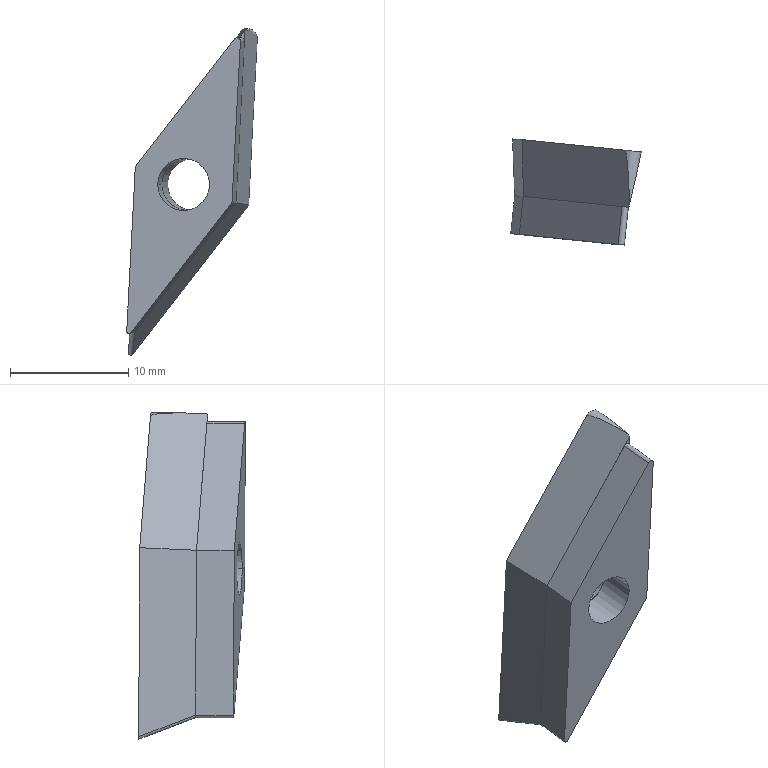Part | Mastercam | 2 solids | 20 faces | box 11.025 x 9.006 x 27.564 mm | volume 930.962 mm3 | plane 12 | cylinder 7 | spline 1 | commonest cylinder face diameters 4.4 x4 0.4 x1 0.6 x1 1.6 x1
STEP:
#1=CARTESIAN_POINT('',(0.,0.,0.));
#2=DIRECTION('',(0.,0.,1.));
#3=DIRECTION('',(1.,0.,0.));
#4=AXIS2_PLACEMENT_3D('',#1,#2,#3);
#5=CARTESIAN_POINT('',(13.05,0.4403,29.477));
#6=VERTEX_POINT('',#5);
#7=CARTESIAN_POINT('',(13.266,0.4177,26.373));
#8=VERTEX_POINT('',#7);
#9=CARTESIAN_POINT('',(11.614,0.5912,27.817));
#10=DIRECTION('',(0.1045,0.9945,0.));
#11=DIRECTION('',(0.7506,-0.07889,-0.6561));
#12=AXIS2_PLACEMENT_3D('',#9,#10,#11);
#13=CIRCLE('',#12,2.2);
#14=EDGE_CURVE('',#6,#8,#13,.T.);
#15=ORIENTED_EDGE('',*,*,#14,.F.);
#16=CARTESIAN_POINT('',(10.179,0.7421,26.156));
#17=VERTEX_POINT('',#16);
#18=CARTESIAN_POINT('',(11.614,0.5912,27.817));
#19=DIRECTION('',(0.1045,0.9945,0.));
#20=DIRECTION('',(0.7506,-0.07889,-0.6561));
#21=AXIS2_PLACEMENT_3D('',#18,#19,#20);
#22=CIRCLE('',#21,2.2);
#23=EDGE_CURVE('',#17,#6,#22,.T.);
#24=ORIENTED_EDGE('',*,*,#23,.F.);
#25=CARTESIAN_POINT('',(11.614,0.5912,27.817));
#26=DIRECTION('',(0.1045,0.9945,0.));
#27=DIRECTION('',(0.7506,-0.07889,-0.6561));
#28=AXIS2_PLACEMENT_3D('',#25,#26,#27);
#29=CIRCLE('',#28,2.2);
#30=EDGE_CURVE('',#8,#17,#29,.T.);
#31=ORIENTED_EDGE('',*,*,#30,.F.);
#32=EDGE_LOOP('',(#15,#24,#31));
#33=FACE_BOUND('',#32,.T.);
#34=CARTESIAN_POINT('',(16.266,0.1023,26.068));
#35=VERTEX_POINT('',#34);
#36=CARTESIAN_POINT('',(6.484,1.13,13.478));
#37=VERTEX_POINT('',#36);
#38=CARTESIAN_POINT('',(24.134,-0.7247,36.194));
#39=DIRECTION('',(-0.6123,0.06435,-0.788));
#40=VECTOR('',#39,1.);
#41=LINE('',#38,#40);
#42=EDGE_CURVE('',#35,#37,#41,.T.);
#43=ORIENTED_EDGE('',*,*,#42,.T.);
#44=CARTESIAN_POINT('',(6.131,1.168,13.611));
#45=VERTEX_POINT('',#44);
#46=CARTESIAN_POINT('',(6.332,1.146,13.609));
#47=DIRECTION('',(0.1045,0.9945,0.));
#48=DIRECTION('',(-0.3483,0.03661,-0.9367));
#49=AXIS2_PLACEMENT_3D('',#46,#47,#48);
#50=ELLIPSE('',#49,0.216,0.2);
#51=EDGE_CURVE('',#37,#45,#50,.T.);
#52=ORIENTED_EDGE('',*,*,#51,.T.);
#53=CARTESIAN_POINT('',(6.963,1.08,29.565));
#54=VERTEX_POINT('',#53);
#55=CARTESIAN_POINT('',(7.647,1.008,42.694));
#56=DIRECTION('',(-0.05205,0.005471,-0.9986));
#57=VECTOR('',#56,1.);
#58=LINE('',#55,#57);
#59=EDGE_CURVE('',#54,#45,#58,.T.);
#60=ORIENTED_EDGE('',*,*,#59,.F.);
#61=CARTESIAN_POINT('',(15.577,0.1747,40.652));
#62=VERTEX_POINT('',#61);
#63=CARTESIAN_POINT('',(16.67,0.05986,42.059));
#64=DIRECTION('',(0.6123,-0.06435,0.788));
#65=VECTOR('',#64,1.);
#66=LINE('',#63,#65);
#67=EDGE_CURVE('',#54,#62,#66,.T.);
#68=ORIENTED_EDGE('',*,*,#67,.T.);
#69=CARTESIAN_POINT('',(16.998,0.02532,40.118));
#70=VERTEX_POINT('',#69);
#71=CARTESIAN_POINT('',(16.204,0.1088,40.159));
#72=DIRECTION('',(-0.1045,-0.9945,0.));
#73=DIRECTION('',(0.6525,-0.06858,0.7547));
#74=AXIS2_PLACEMENT_3D('',#71,#72,#73);
#75=CIRCLE('',#74,0.8);
#76=EDGE_CURVE('',#70,#62,#75,.T.);
#77=ORIENTED_EDGE('',*,*,#76,.F.);
#78=CARTESIAN_POINT('',(17.107,0.01394,42.196));
#79=DIRECTION('',(0.05205,-0.005471,0.9986));
#80=VECTOR('',#79,1.);
#81=LINE('',#78,#80);
#82=EDGE_CURVE('',#35,#70,#81,.T.);
#83=ORIENTED_EDGE('',*,*,#82,.F.);
#84=EDGE_LOOP('',(#43,#52,#60,#68,#77,#83));
#85=FACE_OUTER_BOUND('',#84,.T.);
#86=CARTESIAN_POINT('',(16.451,0.08283,42.23));
#87=DIRECTION('',(-0.1045,-0.9945,0.));
#88=DIRECTION('',(-0.6525,0.06858,-0.7547));
#89=AXIS2_PLACEMENT_3D('',#86,#87,#88);
#90=PLANE('',#89);
#91=ADVANCED_FACE('',(#33,#85),#90,.F.);
#92=CARTESIAN_POINT('',(9.681,-3.992,26.156));
#93=VERTEX_POINT('',#92);
#94=CARTESIAN_POINT('',(9.681,-3.992,26.156));
#95=DIRECTION('',(0.1045,0.9945,0.));
#96=VECTOR('',#95,1.);
#97=LINE('',#94,#96);
#98=EDGE_CURVE('',#93,#17,#97,.T.);
#99=ORIENTED_EDGE('',*,*,#98,.T.);
#100=ORIENTED_EDGE('',*,*,#23,.T.);
#101=CARTESIAN_POINT('',(12.552,-4.294,29.477));
#102=VERTEX_POINT('',#101);
#103=CARTESIAN_POINT('',(12.552,-4.294,29.477));
#104=DIRECTION('',(0.1045,0.9945,0.));
#105=VECTOR('',#104,1.);
#106=LINE('',#103,#105);
#107=EDGE_CURVE('',#102,#6,#106,.T.);
#108=ORIENTED_EDGE('',*,*,#107,.F.);
#109=CARTESIAN_POINT('',(11.117,-4.143,27.817));
#110=DIRECTION('',(0.1045,0.9945,0.));
#111=DIRECTION('',(0.7506,-0.07889,-0.6561));
#112=AXIS2_PLACEMENT_3D('',#109,#110,#111);
#113=CIRCLE('',#112,2.2);
#114=EDGE_CURVE('',#93,#102,#113,.T.);
#115=ORIENTED_EDGE('',*,*,#114,.F.);
#116=EDGE_LOOP('',(#99,#100,#108,#115));
#117=FACE_OUTER_BOUND('',#116,.T.);
#118=CARTESIAN_POINT('',(11.092,-4.379,27.817));
#119=DIRECTION('',(0.1045,0.9945,0.));
#120=DIRECTION('',(0.7506,-0.07889,-0.6561));
#121=AXIS2_PLACEMENT_3D('',#118,#119,#120);
#122=CYLINDRICAL_SURFACE('',#121,2.2);
#123=ADVANCED_FACE('',(#117),#122,.F.);
#124=CARTESIAN_POINT('',(7.036,-3.714,29.351));
#125=VERTEX_POINT('',#124);
#126=CARTESIAN_POINT('',(6.31,-3.638,15.431));
#127=VERTEX_POINT('',#126);
#128=CARTESIAN_POINT('',(7.701,-3.784,42.112));
#129=DIRECTION('',(-0.05205,0.005471,-0.9986));
#130=VECTOR('',#129,1.);
#131=LINE('',#128,#130);
#132=EDGE_CURVE('',#125,#127,#131,.T.);
#133=ORIENTED_EDGE('',*,*,#132,.T.);
#134=CARTESIAN_POINT('',(6.663,-3.675,15.298));
#135=VERTEX_POINT('',#134);
#136=CARTESIAN_POINT('',(6.511,-3.659,15.43));
#137=DIRECTION('',(-0.1045,-0.9945,0.));
#138=DIRECTION('',(-0.3483,0.03661,-0.9367));
#139=AXIS2_PLACEMENT_3D('',#136,#137,#138);
#140=ELLIPSE('',#139,0.216,0.2);
#141=EDGE_CURVE('',#127,#135,#140,.T.);
#142=ORIENTED_EDGE('',*,*,#141,.T.);
#143=CARTESIAN_POINT('',(15.198,-4.572,26.282));
#144=VERTEX_POINT('',#143);
#145=CARTESIAN_POINT('',(15.778,-4.633,27.029));
#146=DIRECTION('',(0.6123,-0.06435,0.788));
#147=VECTOR('',#146,1.);
#148=LINE('',#145,#147);
#149=EDGE_CURVE('',#135,#144,#148,.T.);
#150=ORIENTED_EDGE('',*,*,#149,.T.);
#151=CARTESIAN_POINT('',(15.956,-4.651,40.831));
#152=VERTEX_POINT('',#151);
#153=CARTESIAN_POINT('',(16.,-4.656,41.675));
#154=DIRECTION('',(0.05205,-0.005471,0.9986));
#155=VECTOR('',#154,1.);
#156=LINE('',#153,#155);
#157=EDGE_CURVE('',#144,#152,#156,.T.);
#158=ORIENTED_EDGE('',*,*,#157,.T.);
#159=CARTESIAN_POINT('',(6.51,-3.659,28.674));
#160=DIRECTION('',(-0.6123,0.06435,-0.788));
#161=VECTOR('',#160,1.);
#162=LINE('',#159,#161);
#163=EDGE_CURVE('',#152,#125,#162,.T.);
#164=ORIENTED_EDGE('',*,*,#163,.T.);
#165=EDGE_LOOP('',(#133,#142,#150,#158,#164));
#166=FACE_OUTER_BOUND('',#165,.T.);
#167=CARTESIAN_POINT('',(12.768,-4.316,26.373));
#168=VERTEX_POINT('',#167);
#169=CARTESIAN_POINT('',(11.117,-4.143,27.817));
#170=DIRECTION('',(0.1045,0.9945,0.));
#171=DIRECTION('',(0.7506,-0.07889,-0.6561));
#172=AXIS2_PLACEMENT_3D('',#169,#170,#171);
#173=CIRCLE('',#172,2.2);
#174=EDGE_CURVE('',#168,#93,#173,.T.);
#175=ORIENTED_EDGE('',*,*,#174,.T.);
#176=ORIENTED_EDGE('',*,*,#114,.T.);
#177=CARTESIAN_POINT('',(11.117,-4.143,27.817));
#178=DIRECTION('',(0.1045,0.9945,0.));
#179=DIRECTION('',(0.7506,-0.07889,-0.6561));
#180=AXIS2_PLACEMENT_3D('',#177,#178,#179);
#181=CIRCLE('',#180,2.2);
#182=EDGE_CURVE('',#102,#168,#181,.T.);
#183=ORIENTED_EDGE('',*,*,#182,.T.);
#184=EDGE_LOOP('',(#175,#176,#183));
#185=FACE_BOUND('',#184,.T.);
#186=CARTESIAN_POINT('',(16.265,-4.684,41.661));
#187=DIRECTION('',(-0.1045,-0.9945,0.));
#188=DIRECTION('',(-0.6525,0.06858,-0.7547));
#189=AXIS2_PLACEMENT_3D('',#186,#187,#188);
#190=PLANE('',#189);
#191=ADVANCED_FACE('',(#166,#185),#190,.T.);
#192=ORIENTED_EDGE('',*,*,#149,.F.);
#193=CARTESIAN_POINT('',(6.476,1.343,13.398));
#194=DIRECTION('',(-0.03489,0.9346,-0.3541));
#195=VECTOR('',#194,1.);
#196=LINE('',#193,#195);
#197=EDGE_CURVE('',#135,#37,#196,.T.);
#198=ORIENTED_EDGE('',*,*,#197,.T.);
#199=ORIENTED_EDGE('',*,*,#42,.F.);
#200=CARTESIAN_POINT('',(16.322,0.3479,26.057));
#201=DIRECTION('',(0.2226,0.9739,-0.04472));
#202=VECTOR('',#201,1.);
#203=LINE('',#200,#202);
#204=EDGE_CURVE('',#144,#35,#203,.T.);
#205=ORIENTED_EDGE('',*,*,#204,.F.);
#206=EDGE_LOOP('',(#192,#198,#199,#205));
#207=FACE_OUTER_BOUND('',#206,.T.);
#208=CARTESIAN_POINT('',(16.778,0.2711,26.652));
#209=DIRECTION('',(-0.7651,0.203,0.6111));
#210=DIRECTION('',(-0.6123,0.06435,-0.788));
#211=AXIS2_PLACEMENT_3D('',#208,#209,#210);
#212=PLANE('',#211);
#213=ADVANCED_FACE('',(#207),#212,.F.);
#214=ORIENTED_EDGE('',*,*,#59,.T.);
#215=CARTESIAN_POINT('',(6.302,-3.425,15.351));
#216=DIRECTION('',(0.03489,-0.9346,0.3541));
#217=VECTOR('',#216,1.);
#218=LINE('',#215,#217);
#219=EDGE_CURVE('',#45,#127,#218,.T.);
#220=ORIENTED_EDGE('',*,*,#219,.T.);
#221=ORIENTED_EDGE('',*,*,#132,.F.);
#222=CARTESIAN_POINT('',(7.05,-4.614,29.31));
#223=DIRECTION('',(0.01528,-0.9989,-0.04472));
#224=VECTOR('',#223,1.);
#225=LINE('',#222,#224);
#226=EDGE_CURVE('',#54,#125,#225,.T.);
#227=ORIENTED_EDGE('',*,*,#226,.F.);
#228=EDGE_LOOP('',(#214,#220,#221,#227));
#229=FACE_OUTER_BOUND('',#228,.T.);
#230=CARTESIAN_POINT('',(6.166,-3.878,12.58));
#231=DIRECTION('',(-0.9985,-0.01759,0.05195));
#232=DIRECTION('',(0.05205,-0.005471,0.9986));
#233=AXIS2_PLACEMENT_3D('',#230,#231,#232);
#234=PLANE('',#233);
#235=ADVANCED_FACE('',(#229),#234,.T.);
#236=CARTESIAN_POINT('',(16.006,-4.452,40.909));
#237=VERTEX_POINT('',#236);
#238=CARTESIAN_POINT('',(15.523,-6.371,40.159));
#239=DIRECTION('',(-0.973,0.2248,0.05195));
#240=DIRECTION('',(0.2248,0.9744,-0.006378));
#241=AXIS2_PLACEMENT_3D('',#238,#239,#240);
#242=ELLIPSE('',#241,6.564,0.8);
#243=EDGE_CURVE('',#237,#70,#242,.T.);
#244=ORIENTED_EDGE('',*,*,#243,.F.);
#245=CARTESIAN_POINT('',(15.755,-5.45,40.519));
#246=DIRECTION('',(-0.2284,-0.9069,-0.3541));
#247=VECTOR('',#246,1.);
#248=LINE('',#245,#247);
#249=EDGE_CURVE('',#237,#152,#248,.T.);
#250=ORIENTED_EDGE('',*,*,#249,.T.);
#251=ORIENTED_EDGE('',*,*,#157,.F.);
#252=ORIENTED_EDGE('',*,*,#204,.T.);
#253=ORIENTED_EDGE('',*,*,#82,.T.);
#254=EDGE_LOOP('',(#244,#250,#251,#252,#253));
#255=FACE_OUTER_BOUND('',#254,.T.);
#256=CARTESIAN_POINT('',(15.917,-4.903,41.193));
#257=DIRECTION('',(0.973,-0.2248,-0.05195));
#258=DIRECTION('',(-0.05205,0.005471,-0.9986));
#259=AXIS2_PLACEMENT_3D('',#256,#257,#258);
#260=PLANE('',#259);
#261=ADVANCED_FACE('',(#255),#260,.T.);
#262=ORIENTED_EDGE('',*,*,#249,.F.);
#263=CARTESIAN_POINT('',(15.523,-6.371,40.159));
#264=DIRECTION('',(-0.7906,-0.03945,0.6111));
#265=DIRECTION('',(0.008241,0.9971,0.07503));
#266=AXIS2_PLACEMENT_3D('',#263,#264,#265);
#267=ELLIPSE('',#266,6.564,0.8);
#268=EDGE_CURVE('',#237,#62,#267,.T.);
#269=ORIENTED_EDGE('',*,*,#268,.T.);
#270=ORIENTED_EDGE('',*,*,#67,.F.);
#271=ORIENTED_EDGE('',*,*,#226,.T.);
#272=ORIENTED_EDGE('',*,*,#163,.F.);
#273=EDGE_LOOP('',(#262,#269,#270,#271,#272));
#274=FACE_OUTER_BOUND('',#273,.T.);
#275=CARTESIAN_POINT('',(6.551,1.346,29.051));
#276=DIRECTION('',(0.7906,0.03945,-0.6111));
#277=DIRECTION('',(0.6123,-0.06435,0.788));
#278=AXIS2_PLACEMENT_3D('',#275,#276,#277);
#279=PLANE('',#278);
#280=ADVANCED_FACE('',(#274),#279,.F.);
#281=ORIENTED_EDGE('',*,*,#243,.T.);
#282=ORIENTED_EDGE('',*,*,#76,.T.);
#283=ORIENTED_EDGE('',*,*,#268,.F.);
#284=EDGE_LOOP('',(#281,#282,#283));
#285=FACE_OUTER_BOUND('',#284,.T.);
#286=CARTESIAN_POINT('',(10.977,-49.617,40.159));
#287=DIRECTION('',(0.1045,0.9945,0.));
#288=DIRECTION('',(-0.3483,0.03661,-0.9367));
#289=AXIS2_PLACEMENT_3D('',#286,#287,#288);
#290=CYLINDRICAL_SURFACE('',#289,0.8);
#291=ADVANCED_FACE('',(#285),#290,.T.);
#292=ORIENTED_EDGE('',*,*,#51,.F.);
#293=ORIENTED_EDGE('',*,*,#197,.F.);
#294=ORIENTED_EDGE('',*,*,#141,.F.);
#295=ORIENTED_EDGE('',*,*,#219,.F.);
#296=EDGE_LOOP('',(#292,#293,#294,#295));
#297=FACE_OUTER_BOUND('',#296,.T.);
#298=CARTESIAN_POINT('',(6.482,-2.896,15.141));
#299=DIRECTION('',(-0.03489,0.9346,-0.3541));
#300=DIRECTION('',(0.362,0.3421,0.8672));
#301=AXIS2_PLACEMENT_3D('',#298,#299,#300);
#302=CYLINDRICAL_SURFACE('',#301,0.2);
#303=ADVANCED_FACE('',(#297),#302,.T.);
#304=ORIENTED_EDGE('',*,*,#98,.F.);
#305=ORIENTED_EDGE('',*,*,#174,.F.);
#306=ORIENTED_EDGE('',*,*,#182,.F.);
#307=ORIENTED_EDGE('',*,*,#107,.T.);
#308=ORIENTED_EDGE('',*,*,#14,.T.);
#309=ORIENTED_EDGE('',*,*,#30,.T.);
#310=EDGE_LOOP('',(#304,#305,#306,#307,#308,#309));
#311=FACE_OUTER_BOUND('',#310,.T.);
#312=CARTESIAN_POINT('',(11.092,-4.379,27.817));
#313=DIRECTION('',(0.1045,0.9945,0.));
#314=DIRECTION('',(-0.7506,0.07889,0.6561));
#315=AXIS2_PLACEMENT_3D('',#312,#313,#314);
#316=CYLINDRICAL_SURFACE('',#315,2.2);
#317=ADVANCED_FACE('',(#311),#316,.F.);
#318=CLOSED_SHELL('',(#91,#123,#191,#213,#235,#261,#280,#291,#303,#317));
#319=MANIFOLD_SOLID_BREP('',#318);
#320=CARTESIAN_POINT('',(15.373,-4.59,40.081));
#321=VERTEX_POINT('',#320);
#322=CARTESIAN_POINT('',(7.036,-3.714,29.351));
#323=VERTEX_POINT('',#322);
#324=CARTESIAN_POINT('',(15.373,-4.59,40.081));
#325=DIRECTION('',(-0.6123,0.06435,-0.788));
#326=VECTOR('',#325,1.);
#327=LINE('',#324,#326);
#328=EDGE_CURVE('',#321,#323,#327,.T.);
#329=ORIENTED_EDGE('',*,*,#328,.T.);
#330=CARTESIAN_POINT('',(6.7,-6.906,29.351));
#331=VERTEX_POINT('',#330);
#332=CARTESIAN_POINT('',(6.7,-6.906,29.351));
#333=DIRECTION('',(0.1045,0.9945,0.));
#334=VECTOR('',#333,1.);
#335=LINE('',#332,#334);
#336=EDGE_CURVE('',#331,#323,#335,.T.);
#337=ORIENTED_EDGE('',*,*,#336,.F.);
#338=CARTESIAN_POINT('',(15.038,-7.783,40.081));
#339=VERTEX_POINT('',#338);
#340=CARTESIAN_POINT('',(15.038,-7.783,40.081));
#341=DIRECTION('',(-0.6123,0.06435,-0.788));
#342=VECTOR('',#341,1.);
#343=LINE('',#340,#342);
#344=EDGE_CURVE('',#339,#331,#343,.T.);
#345=ORIENTED_EDGE('',*,*,#344,.F.);
#346=CARTESIAN_POINT('',(15.038,-7.783,40.081));
#347=DIRECTION('',(0.1045,0.9945,0.));
#348=VECTOR('',#347,1.);
#349=LINE('',#346,#348);
#350=EDGE_CURVE('',#339,#321,#349,.T.);
#351=ORIENTED_EDGE('',*,*,#350,.T.);
#352=EDGE_LOOP('',(#329,#337,#345,#351));
#353=FACE_OUTER_BOUND('',#352,.T.);
#354=CARTESIAN_POINT('',(15.038,-7.783,40.081));
#355=DIRECTION('',(0.7837,-0.08237,-0.6157));
#356=DIRECTION('',(-0.6178,0.,-0.7864));
#357=AXIS2_PLACEMENT_3D('',#354,#355,#356);
#358=PLANE('',#357);
#359=ADVANCED_FACE('',(#353),#358,.F.);
#360=CARTESIAN_POINT('',(6.31,-3.638,15.431));
#361=VERTEX_POINT('',#360);
#362=CARTESIAN_POINT('',(7.036,-3.714,29.351));
#363=DIRECTION('',(-0.05205,0.005471,-0.9986));
#364=VECTOR('',#363,1.);
#365=LINE('',#362,#364);
#366=EDGE_CURVE('',#323,#361,#365,.T.);
#367=ORIENTED_EDGE('',*,*,#366,.T.);
#368=CARTESIAN_POINT('',(5.975,-6.83,15.431));
#369=VERTEX_POINT('',#368);
#370=CARTESIAN_POINT('',(5.975,-6.83,15.431));
#371=DIRECTION('',(0.1045,0.9945,0.));
#372=VECTOR('',#371,1.);
#373=LINE('',#370,#372);
#374=EDGE_CURVE('',#369,#361,#373,.T.);
#375=ORIENTED_EDGE('',*,*,#374,.F.);
#376=CARTESIAN_POINT('',(6.7,-6.906,29.351));
#377=DIRECTION('',(-0.05205,0.005471,-0.9986));
#378=VECTOR('',#377,1.);
#379=LINE('',#376,#378);
#380=EDGE_CURVE('',#331,#369,#379,.T.);
#381=ORIENTED_EDGE('',*,*,#380,.F.);
#382=ORIENTED_EDGE('',*,*,#336,.T.);
#383=EDGE_LOOP('',(#367,#375,#381,#382));
#384=FACE_OUTER_BOUND('',#383,.T.);
#385=CARTESIAN_POINT('',(6.7,-6.906,29.351));
#386=DIRECTION('',(0.9932,-0.1044,-0.05234));
#387=DIRECTION('',(0.1045,0.9945,0.));
#388=AXIS2_PLACEMENT_3D('',#385,#386,#387);
#389=PLANE('',#388);
#390=ADVANCED_FACE('',(#384),#389,.F.);
#391=CARTESIAN_POINT('',(6.663,-3.675,15.298));
#392=VERTEX_POINT('',#391);
#393=CARTESIAN_POINT('',(6.31,-3.638,15.431));
#394=CARTESIAN_POINT('',(6.297,-3.636,15.185));
#395=CARTESIAN_POINT('',(6.512,-3.659,15.104));
#396=CARTESIAN_POINT('',(6.663,-3.675,15.298));
#397=(BOUNDED_CURVE()B_SPLINE_CURVE(3,(#393,#394,#395,#396),.UNSPECIFIED.,.F.,.U.)B_SPLINE_CURVE_WITH_KNOTS((4,4),(0.,1.),.UNSPECIFIED.)CURVE()GEOMETRIC_REPRESENTATION_ITEM()RATIONAL_B_SPLINE_CURVE((1.,0.5483,0.5483,1.))REPRESENTATION_ITEM(''));
#398=EDGE_CURVE('',#361,#392,#397,.T.);
#399=ORIENTED_EDGE('',*,*,#398,.T.);
#400=CARTESIAN_POINT('',(6.328,-6.867,15.298));
#401=VERTEX_POINT('',#400);
#402=CARTESIAN_POINT('',(6.328,-6.867,15.298));
#403=DIRECTION('',(0.1045,0.9945,0.));
#404=VECTOR('',#403,1.);
#405=LINE('',#402,#404);
#406=EDGE_CURVE('',#401,#392,#405,.T.);
#407=ORIENTED_EDGE('',*,*,#406,.F.);
#408=CARTESIAN_POINT('',(5.975,-6.83,15.431));
#409=CARTESIAN_POINT('',(5.962,-6.829,15.185));
#410=CARTESIAN_POINT('',(6.176,-6.851,15.104));
#411=CARTESIAN_POINT('',(6.328,-6.867,15.298));
#412=(BOUNDED_CURVE()B_SPLINE_CURVE(3,(#408,#409,#410,#411),.UNSPECIFIED.,.F.,.U.)B_SPLINE_CURVE_WITH_KNOTS((4,4),(0.,1.),.UNSPECIFIED.)CURVE()GEOMETRIC_REPRESENTATION_ITEM()RATIONAL_B_SPLINE_CURVE((1.,0.5483,0.5483,1.))REPRESENTATION_ITEM(''));
#413=EDGE_CURVE('',#369,#401,#412,.T.);
#414=ORIENTED_EDGE('',*,*,#413,.F.);
#415=ORIENTED_EDGE('',*,*,#374,.T.);
#416=EDGE_LOOP('',(#399,#407,#414,#415));
#417=FACE_OUTER_BOUND('',#416,.T.);
#418=CARTESIAN_POINT('',(5.975,-6.83,15.431));
#419=CARTESIAN_POINT('',(6.31,-3.638,15.431));
#420=CARTESIAN_POINT('',(5.962,-6.829,15.185));
#421=CARTESIAN_POINT('',(6.297,-3.636,15.185));
#422=CARTESIAN_POINT('',(6.176,-6.851,15.104));
#423=CARTESIAN_POINT('',(6.512,-3.659,15.104));
#424=CARTESIAN_POINT('',(6.328,-6.867,15.298));
#425=CARTESIAN_POINT('',(6.663,-3.675,15.298));
#426=(BOUNDED_SURFACE()B_SPLINE_SURFACE(3,1,((#418,#419),(#420,#421),(#422,#423),(#424,#425)),.UNSPECIFIED.,.F.,.F.,.U.)B_SPLINE_SURFACE_WITH_KNOTS((4,4),(2,2),(0.,1.),(0.,1.),.UNSPECIFIED.)GEOMETRIC_REPRESENTATION_ITEM()RATIONAL_B_SPLINE_SURFACE(((1.,1.),(0.5483,0.5483),(0.5483,0.5483),(1.,1.)))REPRESENTATION_ITEM('')SURFACE());
#427=ADVANCED_FACE('',(#417),#426,.F.);
#428=CARTESIAN_POINT('',(15.198,-4.572,26.282));
#429=VERTEX_POINT('',#428);
#430=CARTESIAN_POINT('',(6.663,-3.675,15.298));
#431=DIRECTION('',(0.6123,-0.06435,0.788));
#432=VECTOR('',#431,1.);
#433=LINE('',#430,#432);
#434=EDGE_CURVE('',#392,#429,#433,.T.);
#435=ORIENTED_EDGE('',*,*,#434,.T.);
#436=CARTESIAN_POINT('',(14.862,-7.764,26.282));
#437=VERTEX_POINT('',#436);
#438=CARTESIAN_POINT('',(14.862,-7.764,26.282));
#439=DIRECTION('',(0.1045,0.9945,0.));
#440=VECTOR('',#439,1.);
#441=LINE('',#438,#440);
#442=EDGE_CURVE('',#437,#429,#441,.T.);
#443=ORIENTED_EDGE('',*,*,#442,.F.);
#444=CARTESIAN_POINT('',(6.328,-6.867,15.298));
#445=DIRECTION('',(0.6123,-0.06435,0.788));
#446=VECTOR('',#445,1.);
#447=LINE('',#444,#446);
#448=EDGE_CURVE('',#401,#437,#447,.T.);
#449=ORIENTED_EDGE('',*,*,#448,.F.);
#450=ORIENTED_EDGE('',*,*,#406,.T.);
#451=EDGE_LOOP('',(#435,#443,#449,#450));
#452=FACE_OUTER_BOUND('',#451,.T.);
#453=CARTESIAN_POINT('',(6.328,-6.867,15.298));
#454=DIRECTION('',(-0.7837,0.08237,0.6157));
#455=DIRECTION('',(0.6178,0.,0.7864));
#456=AXIS2_PLACEMENT_3D('',#453,#454,#455);
#457=PLANE('',#456);
#458=ADVANCED_FACE('',(#452),#457,.F.);
#459=CARTESIAN_POINT('',(15.906,-4.646,39.881));
#460=VERTEX_POINT('',#459);
#461=CARTESIAN_POINT('',(15.198,-4.572,26.282));
#462=DIRECTION('',(0.05205,-0.005471,0.9986));
#463=VECTOR('',#462,1.);
#464=LINE('',#461,#463);
#465=EDGE_CURVE('',#429,#460,#464,.T.);
#466=ORIENTED_EDGE('',*,*,#465,.T.);
#467=CARTESIAN_POINT('',(15.571,-7.839,39.881));
#468=VERTEX_POINT('',#467);
#469=CARTESIAN_POINT('',(15.571,-7.839,39.881));
#470=DIRECTION('',(0.1045,0.9945,0.));
#471=VECTOR('',#470,1.);
#472=LINE('',#469,#471);
#473=EDGE_CURVE('',#468,#460,#472,.T.);
#474=ORIENTED_EDGE('',*,*,#473,.F.);
#475=CARTESIAN_POINT('',(14.862,-7.764,26.282));
#476=DIRECTION('',(0.05205,-0.005471,0.9986));
#477=VECTOR('',#476,1.);
#478=LINE('',#475,#477);
#479=EDGE_CURVE('',#437,#468,#478,.T.);
#480=ORIENTED_EDGE('',*,*,#479,.F.);
#481=ORIENTED_EDGE('',*,*,#442,.T.);
#482=EDGE_LOOP('',(#466,#474,#480,#481));
#483=FACE_OUTER_BOUND('',#482,.T.);
#484=CARTESIAN_POINT('',(14.862,-7.764,26.282));
#485=DIRECTION('',(-0.9932,0.1044,0.05234));
#486=DIRECTION('',(-0.1045,-0.9945,0.));
#487=AXIS2_PLACEMENT_3D('',#484,#485,#486);
#488=PLANE('',#487);
#489=ADVANCED_FACE('',(#483),#488,.F.);
#490=CARTESIAN_POINT('',(15.608,-4.615,39.896));
#491=DIRECTION('',(-0.1045,-0.9945,0.));
#492=DIRECTION('',(0.9945,-0.1045,0.));
#493=AXIS2_PLACEMENT_3D('',#490,#491,#492);
#494=CIRCLE('',#493,0.3);
#495=EDGE_CURVE('',#460,#321,#494,.T.);
#496=ORIENTED_EDGE('',*,*,#495,.T.);
#497=ORIENTED_EDGE('',*,*,#350,.F.);
#498=CARTESIAN_POINT('',(15.273,-7.807,39.896));
#499=DIRECTION('',(-0.1045,-0.9945,0.));
#500=DIRECTION('',(0.9945,-0.1045,0.));
#501=AXIS2_PLACEMENT_3D('',#498,#499,#500);
#502=CIRCLE('',#501,0.3);
#503=EDGE_CURVE('',#468,#339,#502,.T.);
#504=ORIENTED_EDGE('',*,*,#503,.F.);
#505=ORIENTED_EDGE('',*,*,#473,.T.);
#506=EDGE_LOOP('',(#496,#497,#504,#505));
#507=FACE_OUTER_BOUND('',#506,.T.);
#508=CARTESIAN_POINT('',(15.273,-7.807,39.896));
#509=DIRECTION('',(0.1045,0.9945,0.));
#510=DIRECTION('',(-0.3483,0.03661,-0.9367));
#511=AXIS2_PLACEMENT_3D('',#508,#509,#510);
#512=CYLINDRICAL_SURFACE('',#511,0.3);
#513=ADVANCED_FACE('',(#507),#512,.T.);
#514=CARTESIAN_POINT('',(12.969,-7.565,27.817));
#515=VERTEX_POINT('',#514);
#516=CARTESIAN_POINT('',(13.305,-4.373,27.817));
#517=VERTEX_POINT('',#516);
#518=CARTESIAN_POINT('',(12.969,-7.565,27.817));
#519=DIRECTION('',(0.1045,0.9945,0.));
#520=VECTOR('',#519,1.);
#521=LINE('',#518,#520);
#522=EDGE_CURVE('',#515,#517,#521,.T.);
#523=ORIENTED_EDGE('',*,*,#522,.T.);
#524=CARTESIAN_POINT('',(8.929,-3.913,27.817));
#525=VERTEX_POINT('',#524);
#526=CARTESIAN_POINT('',(11.117,-4.143,27.817));
#527=DIRECTION('',(0.1045,0.9945,0.));
#528=DIRECTION('',(0.9945,-0.1045,0.));
#529=AXIS2_PLACEMENT_3D('',#526,#527,#528);
#530=CIRCLE('',#529,2.2);
#531=EDGE_CURVE('',#517,#525,#530,.T.);
#532=ORIENTED_EDGE('',*,*,#531,.T.);
#533=CARTESIAN_POINT('',(8.593,-7.105,27.817));
#534=VERTEX_POINT('',#533);
#535=CARTESIAN_POINT('',(8.593,-7.105,27.817));
#536=DIRECTION('',(0.1045,0.9945,0.));
#537=VECTOR('',#536,1.);
#538=LINE('',#535,#537);
#539=EDGE_CURVE('',#534,#525,#538,.T.);
#540=ORIENTED_EDGE('',*,*,#539,.F.);
#541=CARTESIAN_POINT('',(10.781,-7.335,27.817));
#542=DIRECTION('',(0.1045,0.9945,0.));
#543=DIRECTION('',(0.9945,-0.1045,0.));
#544=AXIS2_PLACEMENT_3D('',#541,#542,#543);
#545=CIRCLE('',#544,2.2);
#546=EDGE_CURVE('',#515,#534,#545,.T.);
#547=ORIENTED_EDGE('',*,*,#546,.F.);
#548=EDGE_LOOP('',(#523,#532,#540,#547));
#549=FACE_OUTER_BOUND('',#548,.T.);
#550=CARTESIAN_POINT('',(10.781,-7.335,27.817));
#551=DIRECTION('',(0.1045,0.9945,0.));
#552=DIRECTION('',(0.,0.,1.));
#553=AXIS2_PLACEMENT_3D('',#550,#551,#552);
#554=CYLINDRICAL_SURFACE('',#553,2.2);
#555=ADVANCED_FACE('',(#549),#554,.F.);
#556=ORIENTED_EDGE('',*,*,#344,.T.);
#557=ORIENTED_EDGE('',*,*,#380,.T.);
#558=ORIENTED_EDGE('',*,*,#413,.T.);
#559=ORIENTED_EDGE('',*,*,#448,.T.);
#560=ORIENTED_EDGE('',*,*,#479,.T.);
#561=ORIENTED_EDGE('',*,*,#503,.T.);
#562=EDGE_LOOP('',(#556,#557,#558,#559,#560,#561));
#563=FACE_OUTER_BOUND('',#562,.T.);
#564=ORIENTED_EDGE('',*,*,#546,.T.);
#565=CARTESIAN_POINT('',(10.781,-7.335,27.817));
#566=DIRECTION('',(0.1045,0.9945,0.));
#567=DIRECTION('',(0.9945,-0.1045,0.));
#568=AXIS2_PLACEMENT_3D('',#565,#566,#567);
#569=CIRCLE('',#568,2.2);
#570=EDGE_CURVE('',#534,#515,#569,.T.);
#571=ORIENTED_EDGE('',*,*,#570,.T.);
#572=EDGE_LOOP('',(#564,#571));
#573=FACE_BOUND('',#572,.T.);
#574=CARTESIAN_POINT('',(6.1,-6.843,15.228));
#575=DIRECTION('',(0.1045,0.9945,0.));
#576=DIRECTION('',(-0.9945,0.1045,0.));
#577=AXIS2_PLACEMENT_3D('',#574,#575,#576);
#578=PLANE('',#577);
#579=ADVANCED_FACE('',(#563,#573),#578,.F.);
#580=ORIENTED_EDGE('',*,*,#328,.F.);
#581=ORIENTED_EDGE('',*,*,#495,.F.);
#582=ORIENTED_EDGE('',*,*,#465,.F.);
#583=ORIENTED_EDGE('',*,*,#434,.F.);
#584=ORIENTED_EDGE('',*,*,#398,.F.);
#585=ORIENTED_EDGE('',*,*,#366,.F.);
#586=EDGE_LOOP('',(#580,#581,#582,#583,#584,#585));
#587=FACE_OUTER_BOUND('',#586,.T.);
#588=CARTESIAN_POINT('',(11.117,-4.143,27.817));
#589=DIRECTION('',(0.1045,0.9945,0.));
#590=DIRECTION('',(0.9945,-0.1045,0.));
#591=AXIS2_PLACEMENT_3D('',#588,#589,#590);
#592=CIRCLE('',#591,2.2);
#593=EDGE_CURVE('',#525,#517,#592,.T.);
#594=ORIENTED_EDGE('',*,*,#593,.F.);
#595=ORIENTED_EDGE('',*,*,#531,.F.);
#596=EDGE_LOOP('',(#594,#595));
#597=FACE_BOUND('',#596,.T.);
#598=CARTESIAN_POINT('',(6.436,-3.651,15.228));
#599=DIRECTION('',(0.1045,0.9945,0.));
#600=DIRECTION('',(-0.9945,0.1045,0.));
#601=AXIS2_PLACEMENT_3D('',#598,#599,#600);
#602=PLANE('',#601);
#603=ADVANCED_FACE('',(#587,#597),#602,.T.);
#604=ORIENTED_EDGE('',*,*,#522,.F.);
#605=ORIENTED_EDGE('',*,*,#570,.F.);
#606=ORIENTED_EDGE('',*,*,#539,.T.);
#607=ORIENTED_EDGE('',*,*,#593,.T.);
#608=EDGE_LOOP('',(#604,#605,#606,#607));
#609=FACE_OUTER_BOUND('',#608,.T.);
#610=CARTESIAN_POINT('',(10.781,-7.335,27.817));
#611=DIRECTION('',(0.1045,0.9945,0.));
#612=DIRECTION('',(0.,0.,-1.));
#613=AXIS2_PLACEMENT_3D('',#610,#611,#612);
#614=CYLINDRICAL_SURFACE('',#613,2.2);
#615=ADVANCED_FACE('',(#609),#614,.F.);
#616=CLOSED_SHELL('',(#359,#390,#427,#458,#489,#513,#555,#579,#603,#615));
#617=MANIFOLD_SOLID_BREP('',#616);
#618=(LENGTH_UNIT()NAMED_UNIT(*)SI_UNIT(.MILLI.,.METRE.));
#619=UNCERTAINTY_MEASURE_WITH_UNIT(LENGTH_MEASURE(0.005),#618,'','');
#620=(NAMED_UNIT(*)PLANE_ANGLE_UNIT()SI_UNIT($,.RADIAN.));
#621=(GEOMETRIC_REPRESENTATION_CONTEXT(3)GLOBAL_UNCERTAINTY_ASSIGNED_CONTEXT((#619))GLOBAL_UNIT_ASSIGNED_CONTEXT((#618,#620))REPRESENTATION_CONTEXT('',''));
#622=ADVANCED_BREP_SHAPE_REPRESENTATION('',(#4,#319,#617),#621);